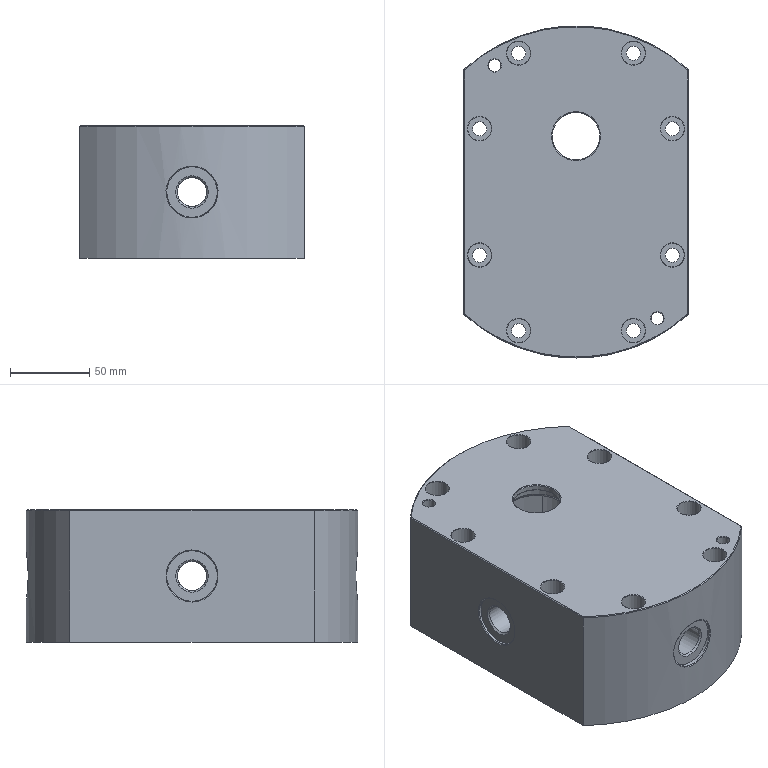NC program | NX | posted with a generic post | part box 142 x 210 x 84 mm
Lines 6739 to 7150 of 7150:
(HOLE_MILLING_COPY_COPY_COPY_COPY , TOOL : D12)
N13434 T12 M6
N13436 G54
N13438 G17 G0 G90 X39.365 Y4.366 B0. C0. S3000 M3
N13440 G43 Z30. H12
N13442 Z-71.5
N13444 G94 G3 X35.25 Y13.9 R5.655 F1500.
N13446 X35.25 Y13.9 Z-71.72 I0. J-13.9
N13448 X35.25 Y13.9 Z-71.94 I0. J-13.9
N13450 X35.25 Y13.9 Z-72.16 I0. J-13.9
N13452 X35.25 Y13.9 Z-72.38 I0. J-13.9
N13454 X35.25 Y13.9 Z-72.6 I0. J-13.9
N13456 X35.25 Y13.9 Z-72.82 I0. J-13.9
N13458 X35.25 Y13.9 Z-73.04 I0. J-13.9
N13460 X35.25 Y13.9 Z-73.26 I0. J-13.9
N13462 X35.25 Y13.9 Z-73.48 I0. J-13.9
N13464 X35.25 Y13.9 Z-73.7 I0. J-13.9
N13466 X35.25 Y13.9 Z-73.92 I0. J-13.9
N13468 X35.25 Y13.9 Z-74.14 I0. J-13.9
N13470 X35.25 Y13.9 Z-74.36 I0. J-13.9
N13472 X35.25 Y13.9 Z-74.58 I0. J-13.9
N13474 X35.25 Y13.9 Z-74.8 I0. J-13.9
N13476 X35.25 Y13.9 Z-75.02 I0. J-13.9
N13478 X35.25 Y13.9 Z-75.24 I0. J-13.9
N13480 X35.25 Y13.9 Z-75.46 I0. J-13.9
N13482 X35.25 Y13.9 Z-75.68 I0. J-13.9
N13484 X35.25 Y13.9 Z-75.9 I0. J-13.9
N13486 X35.25 Y13.9 Z-76.12 I0. J-13.9
N13488 X35.25 Y13.9 Z-76.34 I0. J-13.9
N13490 X35.25 Y13.9 Z-76.56 I0. J-13.9
N13492 X35.25 Y13.9 Z-76.78 I0. J-13.9
N13494 X35.25 Y13.9 Z-77. I0. J-13.9
N13496 X35.25 Y13.9 Z-77.22 I0. J-13.9
N13498 X35.25 Y13.9 Z-77.44 I0. J-13.9
N13500 X35.25 Y13.9 Z-77.66 I0. J-13.9
N13502 X35.25 Y13.9 Z-77.88 I0. J-13.9
N13504 X35.25 Y13.9 Z-78.1 I0. J-13.9
N13506 X35.25 Y13.9 Z-78.32 I0. J-13.9
N13508 X35.25 Y13.9 Z-78.54 I0. J-13.9
N13510 X35.25 Y13.9 Z-78.76 I0. J-13.9
N13512 X35.25 Y13.9 Z-78.98 I0. J-13.9
N13514 X35.25 Y13.9 Z-79.2 I0. J-13.9
N13516 X35.25 Y13.9 Z-79.42 I0. J-13.9
N13518 X35.25 Y13.9 Z-79.64 I0. J-13.9
N13520 X35.25 Y13.9 Z-79.86 I0. J-13.9
N13522 X45.755 Y-9.103 Z-80. R-13.9
N13524 X44.353 Y10.505 R13.9
N13526 X45.755 Y-9.103 R-13.9
N13528 X41.245 Y0.251 R5.655
N13530 G0 Z30.
(FLOOR_WALL_1_COPY , TOOL : D12)
N13532 X-61.726 Y-39.287 S4000
N13534 Z-0.738
N13536 G1 Z-3.738 F500.
N13538 X-59.929 Y-42.4
N13540 G3 X-58.89 Y-43. R1.2
N13542 G1 X58.89 F1000.
N13544 G3 X66.684 Y-38.5 R9.
N13546 X66.684 Y38.5 R77.
N13548 X58.89 Y43. R9.
N13550 G1 X-58.89
N13552 G3 X-66.684 Y38.5 R9.
N13554 X-66.684 Y-38.5 R77.
N13556 X-58.89 Y-43. R9.
N13558 X-57.85 Y-42.4 R1.2
N13560 G1 X-56.465 Y-40.
N13562 Z-0.738
N13564 G0 X-61.726 Y-39.287 Z-10.475
N13566 G1 Z-13.475 F500.
N13568 X-59.929 Y-42.4
N13570 G3 X-58.89 Y-43. R1.2
N13572 G1 X58.89 F1000.
N13574 G3 X66.684 Y-38.5 R9.
N13576 X66.684 Y38.5 R77.
N13578 X58.89 Y43. R9.
N13580 G1 X-58.89
N13582 G3 X-66.684 Y38.5 R9.
N13584 X-66.684 Y-38.5 R77.
N13586 X-58.89 Y-43. R9.
N13588 X-57.85 Y-42.4 R1.2
N13590 G1 X-56.465 Y-40.
N13592 Z-10.475
N13594 G0 X-61.726 Y-39.287 Z-20.213
N13596 G1 Z-23.213 F500.
N13598 X-59.929 Y-42.4
N13600 G3 X-58.89 Y-43. R1.2
N13602 G1 X58.89 F1000.
N13604 G3 X66.684 Y-38.5 R9.
N13606 X66.684 Y38.5 R77.
N13608 X58.89 Y43. R9.
N13610 G1 X-58.89
N13612 G3 X-66.684 Y38.5 R9.
N13614 X-66.684 Y-38.5 R77.
N13616 X-58.89 Y-43. R9.
N13618 X-57.85 Y-42.4 R1.2
N13620 G1 X-56.465 Y-40.
N13622 Z-20.213
N13624 G0 X-61.726 Y-39.287 Z-29.95
N13626 G1 Z-32.95 F500.
N13628 X-59.929 Y-42.4
N13630 G3 X-58.89 Y-43. R1.2
N13632 G1 X58.89 F1000.
N13634 G3 X66.684 Y-38.5 R9.
N13636 X66.684 Y38.5 R77.
N13638 X58.89 Y43. R9.
N13640 G1 X-58.89
N13642 G3 X-66.684 Y38.5 R9.
N13644 X-66.684 Y-38.5 R77.
N13646 X-58.89 Y-43. R9.
N13648 X-57.85 Y-42.4 R1.2
N13650 G1 X-56.465 Y-40.
N13652 Z-29.95
N13654 G0 X-61.726 Y-39.287 Z-39.688
N13656 G1 Z-42.688 F500.
N13658 X-59.929 Y-42.4
N13660 G3 X-58.89 Y-43. R1.2
N13662 G1 X58.89 F1000.
N13664 G3 X66.684 Y-38.5 R9.
N13666 X66.684 Y38.5 R77.
N13668 X58.89 Y43. R9.
N13670 G1 X-58.89
N13672 G3 X-66.684 Y38.5 R9.
N13674 X-66.684 Y-38.5 R77.
N13676 X-58.89 Y-43. R9.
N13678 X-57.85 Y-42.4 R1.2
N13680 G1 X-56.465 Y-40.
N13682 Z-39.688
N13684 G0 X-61.726 Y-39.287 Z-49.425
N13686 G1 Z-52.425 F500.
N13688 X-59.929 Y-42.4
N13690 G3 X-58.89 Y-43. R1.2
N13692 G1 X58.89 F1000.
N13694 G3 X66.684 Y-38.5 R9.
N13696 X66.684 Y38.5 R77.
N13698 X58.89 Y43. R9.
N13700 G1 X-58.89
N13702 G3 X-66.684 Y38.5 R9.
N13704 X-66.684 Y-38.5 R77.
N13706 X-58.89 Y-43. R9.
N13708 X-57.85 Y-42.4 R1.2
N13710 G1 X-56.465 Y-40.
N13712 Z-49.425
N13714 G0 X-61.726 Y-39.287 Z-59.163
N13716 G1 Z-62.163 F500.
N13718 X-59.929 Y-42.4
N13720 G3 X-58.89 Y-43. R1.2
N13722 G1 X58.89 F1000.
N13724 G3 X66.684 Y-38.5 R9.
N13726 X66.684 Y38.5 R77.
N13728 X58.89 Y43. R9.
N13730 G1 X-58.89
N13732 G3 X-66.684 Y38.5 R9.
N13734 X-66.684 Y-38.5 R77.
N13736 X-58.89 Y-43. R9.
N13738 X-57.85 Y-42.4 R1.2
N13740 G1 X-56.465 Y-40.
N13742 Z-59.163
N13744 G0 X-61.726 Y-39.287 Z-68.9
N13746 G1 Z-71.9 F500.
N13748 X-59.929 Y-42.4
N13750 G3 X-58.89 Y-43. R1.2
N13752 G1 X58.89 F1000.
N13754 G3 X66.684 Y-38.5 R9.
N13756 X66.684 Y38.5 R77.
N13758 X58.89 Y43. R9.
N13760 G1 X-58.89
N13762 G3 X-66.684 Y38.5 R9.
N13764 X-66.684 Y-38.5 R77.
N13766 X-58.89 Y-43. R9.
N13768 X-57.85 Y-42.4 R1.2
N13770 G1 X-56.465 Y-40.
N13772 Z-68.9
N13774 G0 Z30.
(FLOOR_WALL_1_COPY_COPY , TOOL : D12)
N13776 X-57.98 Y41.799
N13778 Z-69.
N13780 G1 Z-72. F500.
N13782 G3 X-59.019 Y42.399 R1.2
N13784 G1 X59.019 F1000.
N13786 G2 X66.164 Y38.2 R8.4
N13788 X66.983 Y36.746 R76.4
N13790 G1 X-66.983
N13792 G3 X-69.787 Y31.092 R76.4
N13794 G1 X69.787
N13796 G2 X72.04 Y25.439 R76.4
N13798 G1 X-72.04
N13800 G3 X-73.793 Y19.786 R76.4
N13802 G1 X73.793
N13804 G2 X75.081 Y14.133 R76.4
N13806 G1 X-75.081
N13808 G3 X-75.928 Y8.479 R76.4
N13810 G1 X75.928
N13812 G2 X76.348 Y2.826 R76.4
N13814 G1 X-76.348
N13816 G3 X-76.348 Y-2.827 R76.4
N13818 G1 X76.348
N13820 G2 X75.928 Y-8.48 R76.4
N13822 G1 X-75.928
N13824 G3 X-75.081 Y-14.134 R76.4
N13826 G1 X75.081
N13828 G2 X73.793 Y-19.787 R76.4
N13830 G1 X-73.793
N13832 G3 X-72.04 Y-25.44 R76.4
N13834 G1 X72.04
N13836 G2 X69.787 Y-31.093 R76.4
N13838 G1 X-69.787
N13840 G3 X-66.982 Y-36.747 R76.4
N13842 G1 X66.982
N13844 G2 X66.164 Y-38.2 R76.4
N13846 X58.903 Y-42.4 R8.4
N13848 G1 X-58.903
N13850 G2 X-59.942 Y-41.8 R1.2
N13852 G1 Y-42.398
N13854 G3 X-58.903 Y-43. R1.2 F500.
N13856 G1 X58.89 F1000.
N13858 G3 X66.684 Y-38.5 R9.
N13860 X66.684 Y38.5 R77.
N13862 X58.89 Y43. R9.
N13864 G1 X-58.89
N13866 G3 X-66.684 Y38.5 R9.
N13868 X-66.684 Y-38.5 R77.
N13870 X-58.903 Y-43. R9.
N13872 X-57.863 Y-42.402 R1.2
N13874 G1 X-56.472 Y-40.
N13876 Z-69.
N13878 G0 Z30.
N13880 M5
(PLANAR_MILL_COPY_COPY_COPY , TOOL : D6A45)
N13882 T07 M6
N13884 G54
N13886 G17 G0 G90 X39.234 Y-63.843 B0. C0. S7500 M3
N13888 G43 Z30. H7
N13890 Z1.5
N13892 G94 G1 Z-1.5 F1250.
N13894 G3 X40. Y-64.2 R1.
N13896 X43.2 Y-61. R3.2
N13898 X40. Y-64.2 R-3.2
N13900 X40.766 Y-63.843 R1.
N13902 G1 Z1.5
N13904 G0 Z30.
N13906 X79.234 Y-53.843
N13908 Z1.5
N13910 G1 Z-1.5
N13912 G3 X80. Y-54.2 R1.
N13914 X82.7 Y-51.5 R2.7
N13916 X80. Y-54.2 R-2.7
N13918 X80.766 Y-53.843 R1.
N13920 G1 Z1.5
N13922 G0 Z30.
N13924 X90.611 Y-37.121
N13926 Z1.5
N13928 G1 Z-1.5
N13930 G3 X90.969 Y-36.355 R1.
N13932 X87.769 Y-33.155 R3.2
N13934 X90.969 Y-36.355 R-3.2
N13936 X90.611 Y-35.589 R1.
N13938 G1 Z1.5
N13940 G0 Z30.
N13942 Y35.589
N13944 Z1.5
N13946 G1 Z-1.5
N13948 G3 X90.969 Y36.355 R1.
N13950 X87.769 Y39.555 R3.2
N13952 X90.969 Y36.355 R-3.2
N13954 X90.611 Y37.121 R1.
N13956 G1 Z1.5
N13958 G0 Z30.
N13960 X40.766 Y63.843
N13962 Z1.5
N13964 G1 Z-1.5
N13966 G3 X40. Y64.2 R1.
N13968 X36.8 Y61. R3.2
N13970 X40. Y64.2 R-3.2
N13972 X39.234 Y63.843 R1.
N13974 G1 Z1.5
N13976 G0 Z30.
N13978 X0.766 Y47.343
N13980 Z1.5
N13982 G1 Z-1.5
N13984 G3 X0. Y47.7 R1.
N13986 G1 X-58.89
N13988 G3 X-70.754 Y40.85 R13.7
N13990 X-70.754 Y-40.85 R81.7
N13992 X-58.89 Y-47.7 R13.7
N13994 G1 X58.89
N13996 G3 X70.754 Y-40.85 R13.7
N13998 X70.754 Y40.85 R81.7
N14000 X58.89 Y47.7 R13.7
N14002 G1 X0.
N14004 G3 X-0.766 Y47.343 R1.
N14006 G1 Z1.5
N14008 G0 Z30.
N14010 X0.766 Y53.343
N14012 Z1.5
N14014 G1 Z-1.5
N14016 G3 X0. Y53.7 R1.
N14018 G1 X-58.89
N14020 G3 X-75.95 Y43.85 R19.7
N14022 X-75.95 Y-43.85 R87.7
N14024 X-58.89 Y-53.7 R19.7
N14026 G1 X58.89
N14028 G3 X75.95 Y-43.85 R19.7
N14030 X75.95 Y43.85 R87.7
N14032 X58.89 Y53.7 R19.7
N14034 G1 X0.
N14036 G3 X-0.766 Y53.343 R1.
N14038 G1 Z1.5
N14040 G0 Z30.
N14042 Y53.657
N14044 Z1.5
N14046 G1 Z-1.5
N14048 G3 X0. Y53.3 R1.
N14050 G1 X58.89
N14052 G2 X75.604 Y43.65 R19.3
N14054 X75.604 Y-43.65 R87.3
N14056 X58.89 Y-53.3 R19.3
N14058 G1 X-58.89
N14060 G2 X-75.604 Y-43.65 R19.3
N14062 X-75.604 Y43.65 R87.3
N14064 X-58.89 Y53.3 R19.3
N14066 G1 X0.
N14068 G3 X0.766 Y53.657 R1.
N14070 G1 Z1.5
N14072 G0 Z30.
N14074 X-0.766 Y72.657
N14076 Z1.5
N14078 G1 Z-1.5
N14080 G3 X0. Y72.3 R1.
N14082 G1 X77.356
N14084 G2 X78.314 Y71.879 R1.3
N14086 X78.314 Y-71.879 R106.3
N14088 X77.356 Y-72.3 R1.3
N14090 G1 X-77.356
N14092 G2 X-78.314 Y-71.879 R1.3
N14094 X-78.314 Y71.879 R106.3
N14096 X-77.356 Y72.3 R1.3
N14098 G1 X0.
N14100 G3 X0.766 Y72.657 R1.
N14102 G1 Z1.5
N14104 G0 Z30.
N14106 X-39.234 Y63.843
N14108 Z1.5
N14110 G1 Z-1.5
N14112 G3 X-40. Y64.2 R1.
N14114 X-43.2 Y61. R3.2
N14116 X-40. Y64.2 R-3.2
N14118 X-40.766 Y63.843 R1.
N14120 G1 Z1.5
N14122 G0 Z30.
N14124 X-79.234 Y53.843
N14126 Z1.5
N14128 G1 Z-1.5
N14130 G3 X-80. Y54.2 R1.
N14132 X-82.7 Y51.5 R2.7
N14134 X-80. Y54.2 R-2.7
N14136 X-80.766 Y53.843 R1.
N14138 G1 Z1.5
N14140 G0 Z30.
N14142 X-90.611 Y37.121
N14144 Z1.5
N14146 G1 Z-1.5
N14148 G3 X-90.969 Y36.355 R1.
N14150 X-87.769 Y33.155 R3.2
N14152 X-90.969 Y36.355 R-3.2
N14154 X-90.611 Y35.589 R1.
N14156 G1 Z1.5
N14158 G0 Z30.
N14160 Y-35.589
N14162 Z1.5
N14164 G1 Z-1.5
N14166 G3 X-90.969 Y-36.355 R1.
N14168 X-87.769 Y-39.555 R3.2
N14170 X-90.969 Y-36.355 R-3.2
N14172 X-90.611 Y-37.121 R1.
N14174 G1 Z1.5
N14176 G0 Z30.
N14178 X-40.766 Y-63.843
N14180 Z1.5
N14182 G1 Z-1.5
N14184 G3 X-40. Y-64.2 R1.
N14186 X-36.8 Y-61. R3.2
N14188 X-40. Y-64.2 R-3.2
N14190 X-39.234 Y-63.843 R1.
N14192 G1 Z1.5
N14194 G0 Z30.
N14196 M5
(CUTTERCOMP12 , TOOL : D12)
N14198 T12 M6
N14200 G54
N14202 G17 G0 G90 X38.343 Y10.348 B0. C0. S4000 M3
N14204 G43 Z30. H12
N14206 Z-80.
N14208 G41 G94 G1 X38.372 Y10.443 F1000. D12
N14210 G3 X35.25 Y13.95 R3.143
N14212 X21.3 Y0. R13.95
N14214 X35.25 Y13.95 R-13.95
N14216 X32.128 Y10.443 R3.143
N14218 G40
N14220 G1 X32.157 Y10.348
N14222 G0 Z30.
N14224 M5
N14226 M2